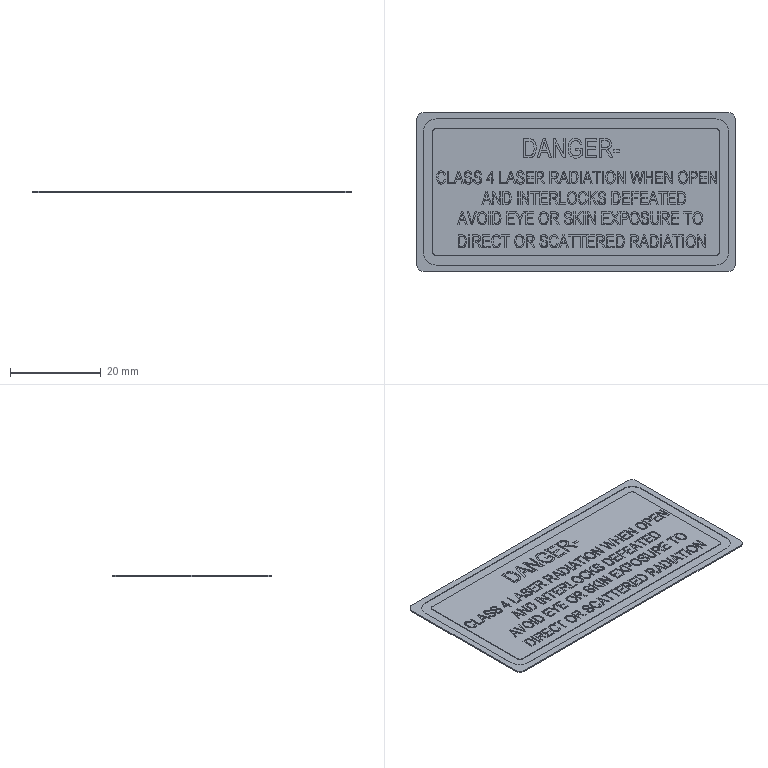Part | STEP file | BBS-JG-IEC-L70X35-2.stp.STEP | 1 solid | 1877 faces | box 70 x 35 x 0.28 mm | volume 599.618 mm3 | plane 978 | spline 887 | cylinder 12 | commonest cylinder face diameters 1.4 x4 2.8 x4 5.6 x4